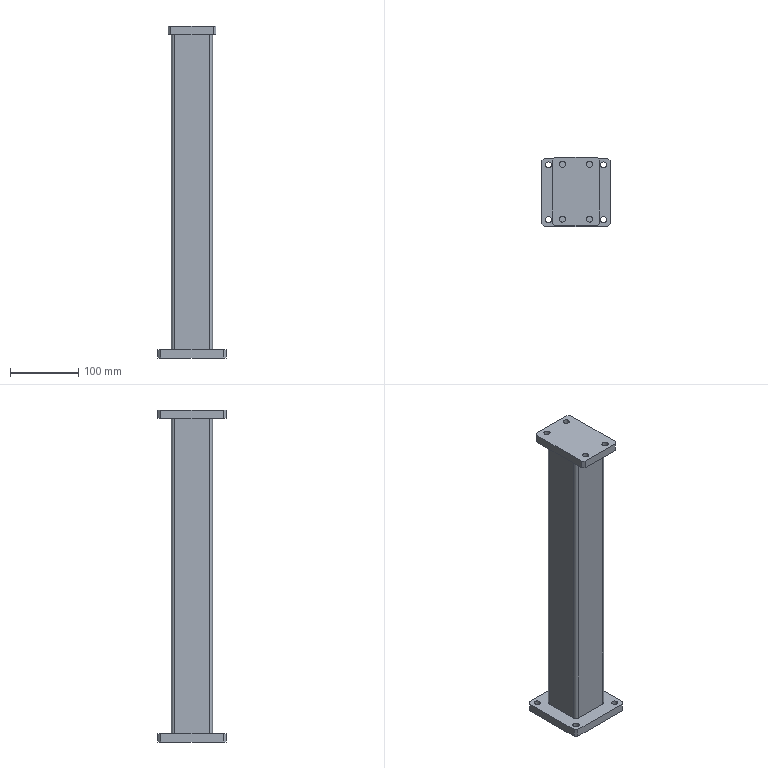Part | STEP file | Cable Fixing Bracket | 1 solid | 54 faces | box 100 x 100 x 485 mm | volume 512449 mm3 | plane 30 | cylinder 24 | commonest cylinder face diameters 9 x16 10 x8